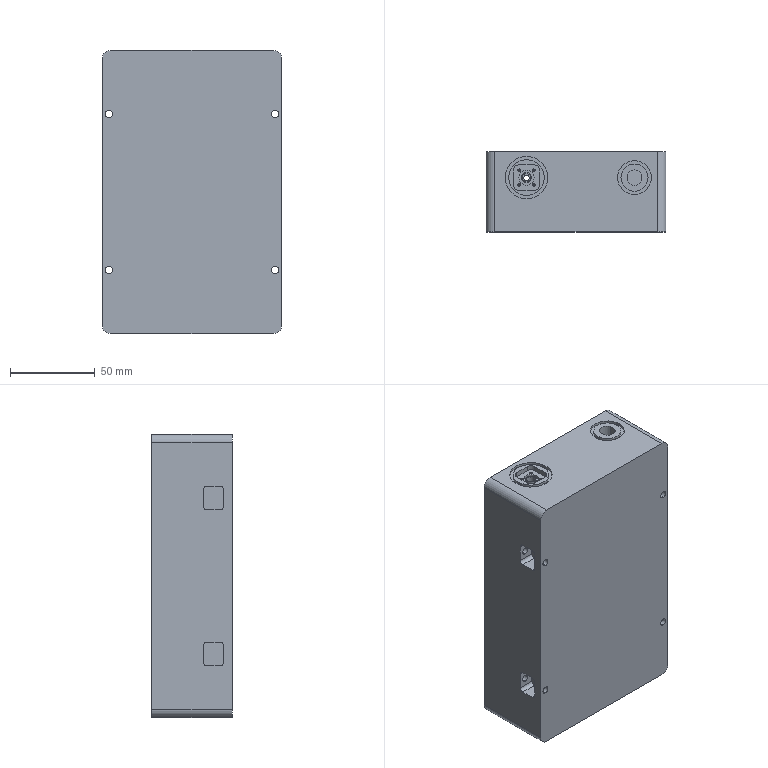Part | SolidWorks | features ICE 29, MoveFace 24, HoleWzd 23, Fillet 19, Cut 18, DelFace 18, 3DProfileFeature 1, Extrusion 1, LPattern 1 | 1 solid | 476 faces | box 106 x 47.3 x 167 mm | volume 437913 mm3 | cylinder 253 | cone 132 | plane 91 | commonest cylinder face diameters 2.5 x90 6 x43 3.3 x26 1.6 x20 4 x16 4.2 x16